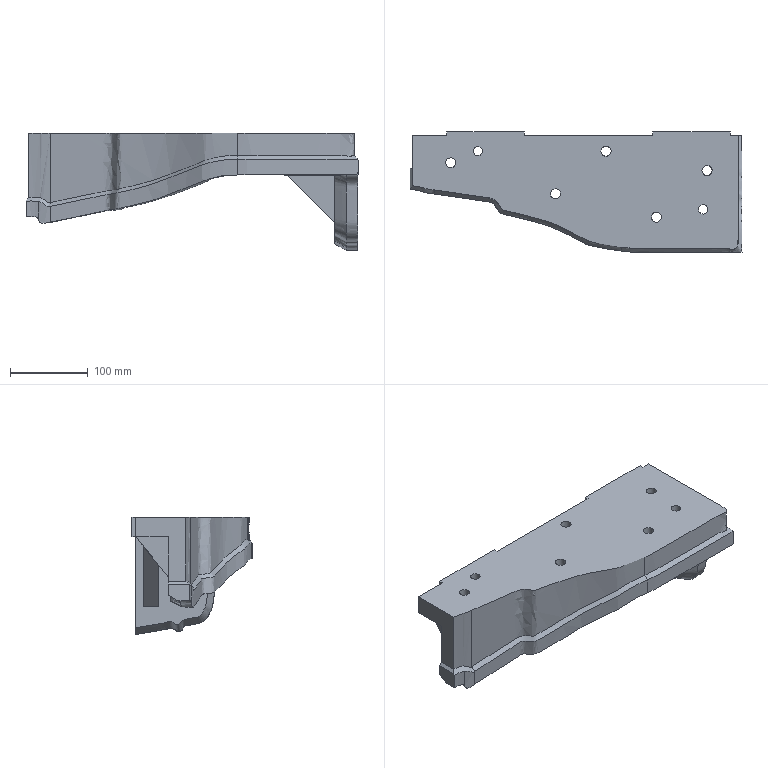Part | NX | features solid 2 | 1 solid | 75 faces | box 427.317 x 155.091 x 150.732 mm | volume 2219618 mm3 | plane 39 | spline 18 | cylinder 16 | cone 2 | commonest cylinder face diameters 13 x7 30 x7 12 x2